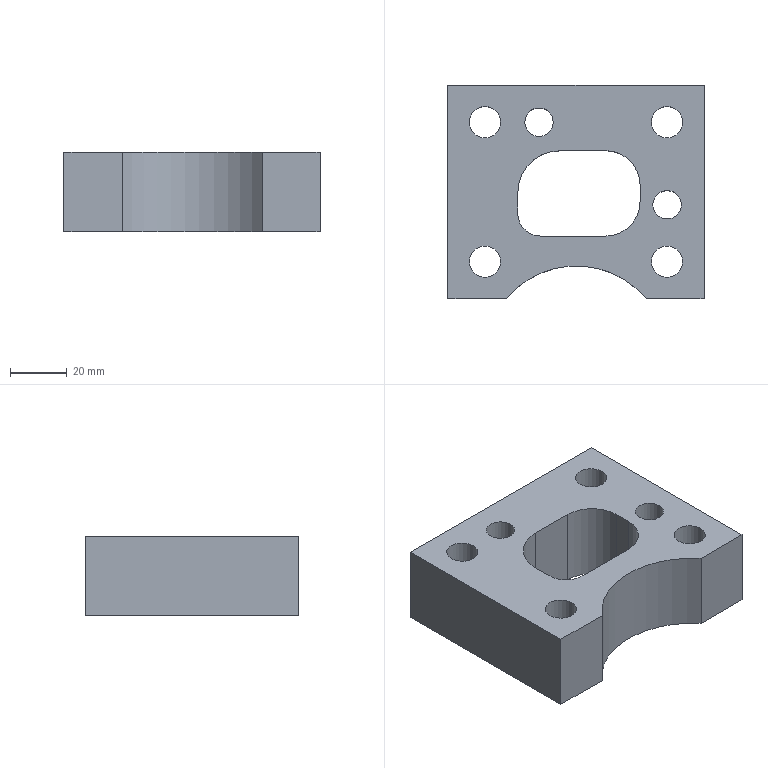Part | STEP file | PN_0017_id886_x_t | 1 solid | 30 faces | box 90 x 75 x 28 mm | volume 120807 mm3 | plane 15 | cylinder 15 | commonest cylinder face diameters 11 x4 17 x4 10 x2 24 x2 16 x1 30 x1
STEP:
#1=CARTESIAN_POINT('',(-240.086,-141.5,67.));
#2=VERTEX_POINT('',#1);
#3=CARTESIAN_POINT('',(-219.571,-141.5,67.));
#4=VERTEX_POINT('',#3);
#5=CARTESIAN_POINT('',(-207.586,-141.5,67.));
#6=DIRECTION('',(1.,0.,0.));
#7=VECTOR('',#6,1.);
#8=LINE('',#5,#7);
#9=EDGE_CURVE('',#2,#4,#8,.T.);
#10=ORIENTED_EDGE('',*,*,#9,.T.);
#11=CARTESIAN_POINT('',(-219.571,-141.5,95.));
#12=VERTEX_POINT('',#11);
#13=CARTESIAN_POINT('',(-219.571,-141.5,96.5));
#14=DIRECTION('',(0.,0.,-1.));
#15=VECTOR('',#14,1.);
#16=LINE('',#13,#15);
#17=EDGE_CURVE('',#12,#4,#16,.T.);
#18=ORIENTED_EDGE('',*,*,#17,.F.);
#19=CARTESIAN_POINT('',(-240.086,-141.5,95.));
#20=VERTEX_POINT('',#19);
#21=CARTESIAN_POINT('',(-207.586,-141.5,95.));
#22=DIRECTION('',(-1.,0.,0.));
#23=VECTOR('',#22,1.);
#24=LINE('',#21,#23);
#25=EDGE_CURVE('',#12,#20,#24,.T.);
#26=ORIENTED_EDGE('',*,*,#25,.T.);
#27=CARTESIAN_POINT('',(-240.086,-141.5,77.));
#28=DIRECTION('',(0.,0.,1.));
#29=VECTOR('',#28,1.);
#30=LINE('',#27,#29);
#31=EDGE_CURVE('',#2,#20,#30,.T.);
#32=ORIENTED_EDGE('',*,*,#31,.F.);
#33=EDGE_LOOP('',(#10,#18,#26,#32));
#34=FACE_OUTER_BOUND('',#33,.T.);
#35=CARTESIAN_POINT('',(-207.586,-141.5,77.));
#36=DIRECTION('',(0.,-1.,0.));
#37=DIRECTION('',(0.,0.,-1.));
#38=AXIS2_PLACEMENT_3D('',#35,#36,#37);
#39=PLANE('',#38);
#40=ADVANCED_FACE('',(#34),#39,.T.);
#41=CARTESIAN_POINT('',(-221.586,-79.5,95.));
#42=VERTEX_POINT('',#41);
#43=CARTESIAN_POINT('',(-227.086,-79.5,95.));
#44=DIRECTION('',(0.,0.,1.));
#45=DIRECTION('',(1.,0.,0.));
#46=AXIS2_PLACEMENT_3D('',#43,#44,#45);
#47=CIRCLE('',#46,5.5);
#48=EDGE_CURVE('',#42,#42,#47,.T.);
#49=ORIENTED_EDGE('',*,*,#48,.F.);
#50=EDGE_LOOP('',(#49));
#51=FACE_BOUND('',#50,.T.);
#52=CARTESIAN_POINT('',(-157.586,-79.5,95.));
#53=VERTEX_POINT('',#52);
#54=CARTESIAN_POINT('',(-163.086,-79.5,95.));
#55=DIRECTION('',(0.,0.,1.));
#56=DIRECTION('',(1.,0.,0.));
#57=AXIS2_PLACEMENT_3D('',#54,#55,#56);
#58=CIRCLE('',#57,5.5);
#59=EDGE_CURVE('',#53,#53,#58,.T.);
#60=ORIENTED_EDGE('',*,*,#59,.F.);
#61=EDGE_LOOP('',(#60));
#62=FACE_BOUND('',#61,.T.);
#63=CARTESIAN_POINT('',(-221.586,-128.5,95.));
#64=VERTEX_POINT('',#63);
#65=CARTESIAN_POINT('',(-227.086,-128.5,95.));
#66=DIRECTION('',(0.,0.,1.));
#67=DIRECTION('',(1.,0.,0.));
#68=AXIS2_PLACEMENT_3D('',#65,#66,#67);
#69=CIRCLE('',#68,5.5);
#70=EDGE_CURVE('',#64,#64,#69,.T.);
#71=ORIENTED_EDGE('',*,*,#70,.F.);
#72=EDGE_LOOP('',(#71));
#73=FACE_BOUND('',#72,.T.);
#74=CARTESIAN_POINT('',(-157.586,-128.5,95.));
#75=VERTEX_POINT('',#74);
#76=CARTESIAN_POINT('',(-163.086,-128.5,95.));
#77=DIRECTION('',(0.,0.,1.));
#78=DIRECTION('',(1.,0.,0.));
#79=AXIS2_PLACEMENT_3D('',#76,#77,#78);
#80=CIRCLE('',#79,5.5);
#81=EDGE_CURVE('',#75,#75,#80,.T.);
#82=ORIENTED_EDGE('',*,*,#81,.F.);
#83=EDGE_LOOP('',(#82));
#84=FACE_BOUND('',#83,.T.);
#85=CARTESIAN_POINT('',(-170.429,-141.5,95.));
#86=VERTEX_POINT('',#85);
#87=CARTESIAN_POINT('',(-195.,-162.,95.));
#88=DIRECTION('',(0.,0.,1.));
#89=DIRECTION('',(1.,0.,0.));
#90=AXIS2_PLACEMENT_3D('',#87,#88,#89);
#91=CIRCLE('',#90,32.);
#92=EDGE_CURVE('',#86,#12,#91,.T.);
#93=ORIENTED_EDGE('',*,*,#92,.F.);
#94=CARTESIAN_POINT('',(-150.086,-141.5,95.));
#95=VERTEX_POINT('',#94);
#96=CARTESIAN_POINT('',(-207.586,-141.5,95.));
#97=DIRECTION('',(-1.,0.,0.));
#98=VECTOR('',#97,1.);
#99=LINE('',#96,#98);
#100=EDGE_CURVE('',#95,#86,#99,.T.);
#101=ORIENTED_EDGE('',*,*,#100,.F.);
#102=CARTESIAN_POINT('',(-150.086,-66.5,95.));
#103=VERTEX_POINT('',#102);
#104=CARTESIAN_POINT('',(-150.086,-99.,95.));
#105=DIRECTION('',(0.,-1.,0.));
#106=VECTOR('',#105,1.);
#107=LINE('',#104,#106);
#108=EDGE_CURVE('',#103,#95,#107,.T.);
#109=ORIENTED_EDGE('',*,*,#108,.F.);
#110=CARTESIAN_POINT('',(-240.086,-66.5,95.));
#111=VERTEX_POINT('',#110);
#112=CARTESIAN_POINT('',(-207.586,-66.5,95.));
#113=DIRECTION('',(1.,0.,0.));
#114=VECTOR('',#113,1.);
#115=LINE('',#112,#114);
#116=EDGE_CURVE('',#111,#103,#115,.T.);
#117=ORIENTED_EDGE('',*,*,#116,.F.);
#118=CARTESIAN_POINT('',(-240.086,-99.,95.));
#119=DIRECTION('',(0.,1.,0.));
#120=VECTOR('',#119,1.);
#121=LINE('',#118,#120);
#122=EDGE_CURVE('',#20,#111,#121,.T.);
#123=ORIENTED_EDGE('',*,*,#122,.F.);
#124=ORIENTED_EDGE('',*,*,#25,.F.);
#125=EDGE_LOOP('',(#93,#101,#109,#117,#123,#124));
#126=FACE_BOUND('',#125,.T.);
#127=CARTESIAN_POINT('',(-184.586,-119.5,95.));
#128=VERTEX_POINT('',#127);
#129=CARTESIAN_POINT('',(-172.586,-107.5,95.));
#130=VERTEX_POINT('',#129);
#131=CARTESIAN_POINT('',(-184.586,-107.5,95.));
#132=DIRECTION('',(0.,0.,1.));
#133=DIRECTION('',(-1.,0.,0.));
#134=AXIS2_PLACEMENT_3D('',#131,#132,#133);
#135=CIRCLE('',#134,12.);
#136=EDGE_CURVE('',#128,#130,#135,.T.);
#137=ORIENTED_EDGE('',*,*,#136,.F.);
#138=CARTESIAN_POINT('',(-207.586,-119.5,95.));
#139=VERTEX_POINT('',#138);
#140=CARTESIAN_POINT('',(-211.586,-119.5,95.));
#141=DIRECTION('',(1.,0.,0.));
#142=VECTOR('',#141,1.);
#143=LINE('',#140,#142);
#144=EDGE_CURVE('',#139,#128,#143,.T.);
#145=ORIENTED_EDGE('',*,*,#144,.F.);
#146=CARTESIAN_POINT('',(-215.586,-111.5,95.));
#147=VERTEX_POINT('',#146);
#148=CARTESIAN_POINT('',(-207.586,-111.5,95.));
#149=DIRECTION('',(0.,0.,1.));
#150=DIRECTION('',(-1.,0.,0.));
#151=AXIS2_PLACEMENT_3D('',#148,#149,#150);
#152=CIRCLE('',#151,8.);
#153=EDGE_CURVE('',#147,#139,#152,.T.);
#154=ORIENTED_EDGE('',*,*,#153,.F.);
#155=CARTESIAN_POINT('',(-215.586,-104.5,95.));
#156=VERTEX_POINT('',#155);
#157=CARTESIAN_POINT('',(-215.586,-80.,95.));
#158=DIRECTION('',(0.,-1.,0.));
#159=VECTOR('',#158,1.);
#160=LINE('',#157,#159);
#161=EDGE_CURVE('',#156,#147,#160,.T.);
#162=ORIENTED_EDGE('',*,*,#161,.F.);
#163=CARTESIAN_POINT('',(-200.586,-89.5,95.));
#164=VERTEX_POINT('',#163);
#165=CARTESIAN_POINT('',(-200.586,-104.5,95.));
#166=DIRECTION('',(0.,0.,1.));
#167=DIRECTION('',(-1.,0.,0.));
#168=AXIS2_PLACEMENT_3D('',#165,#166,#167);
#169=CIRCLE('',#168,15.);
#170=EDGE_CURVE('',#164,#156,#169,.T.);
#171=ORIENTED_EDGE('',*,*,#170,.F.);
#172=CARTESIAN_POINT('',(-184.586,-89.5,95.));
#173=VERTEX_POINT('',#172);
#174=CARTESIAN_POINT('',(-189.586,-89.5,95.));
#175=DIRECTION('',(-1.,0.,0.));
#176=VECTOR('',#175,1.);
#177=LINE('',#174,#176);
#178=EDGE_CURVE('',#173,#164,#177,.T.);
#179=ORIENTED_EDGE('',*,*,#178,.F.);
#180=CARTESIAN_POINT('',(-172.586,-101.5,95.));
#181=VERTEX_POINT('',#180);
#182=CARTESIAN_POINT('',(-184.586,-101.5,95.));
#183=DIRECTION('',(0.,0.,1.));
#184=DIRECTION('',(-1.,0.,0.));
#185=AXIS2_PLACEMENT_3D('',#182,#183,#184);
#186=CIRCLE('',#185,12.);
#187=EDGE_CURVE('',#181,#173,#186,.T.);
#188=ORIENTED_EDGE('',*,*,#187,.F.);
#189=CARTESIAN_POINT('',(-172.586,-115.,95.));
#190=DIRECTION('',(0.,1.,0.));
#191=VECTOR('',#190,1.);
#192=LINE('',#189,#191);
#193=EDGE_CURVE('',#130,#181,#192,.T.);
#194=ORIENTED_EDGE('',*,*,#193,.F.);
#195=EDGE_LOOP('',(#137,#145,#154,#162,#171,#179,#188,#194));
#196=FACE_BOUND('',#195,.T.);
#197=CARTESIAN_POINT('',(-168.086,-108.5,95.));
#198=VERTEX_POINT('',#197);
#199=CARTESIAN_POINT('',(-163.086,-108.5,95.));
#200=DIRECTION('',(0.,0.,1.));
#201=DIRECTION('',(-1.,0.,0.));
#202=AXIS2_PLACEMENT_3D('',#199,#200,#201);
#203=CIRCLE('',#202,5.);
#204=EDGE_CURVE('',#198,#198,#203,.T.);
#205=ORIENTED_EDGE('',*,*,#204,.F.);
#206=EDGE_LOOP('',(#205));
#207=FACE_BOUND('',#206,.T.);
#208=CARTESIAN_POINT('',(-203.086,-79.5,95.));
#209=VERTEX_POINT('',#208);
#210=CARTESIAN_POINT('',(-208.086,-79.5,95.));
#211=DIRECTION('',(0.,0.,1.));
#212=DIRECTION('',(1.,0.,0.));
#213=AXIS2_PLACEMENT_3D('',#210,#211,#212);
#214=CIRCLE('',#213,5.);
#215=EDGE_CURVE('',#209,#209,#214,.T.);
#216=ORIENTED_EDGE('',*,*,#215,.F.);
#217=EDGE_LOOP('',(#216));
#218=FACE_BOUND('',#217,.T.);
#219=CARTESIAN_POINT('',(-119.811,64.,95.));
#220=DIRECTION('',(0.,0.,1.));
#221=DIRECTION('',(1.,0.,0.));
#222=AXIS2_PLACEMENT_3D('',#219,#220,#221);
#223=PLANE('',#222);
#224=ADVANCED_FACE('',(#51,#62,#73,#84,#126,#196,#207,#218),#223,.T.);
#225=CARTESIAN_POINT('',(-170.429,-141.5,67.));
#226=VERTEX_POINT('',#225);
#227=CARTESIAN_POINT('',(-170.429,-141.5,96.5));
#228=DIRECTION('',(0.,0.,1.));
#229=VECTOR('',#228,1.);
#230=LINE('',#227,#229);
#231=EDGE_CURVE('',#226,#86,#230,.T.);
#232=ORIENTED_EDGE('',*,*,#231,.F.);
#233=CARTESIAN_POINT('',(-150.086,-141.5,67.));
#234=VERTEX_POINT('',#233);
#235=CARTESIAN_POINT('',(-207.586,-141.5,67.));
#236=DIRECTION('',(1.,0.,0.));
#237=VECTOR('',#236,1.);
#238=LINE('',#235,#237);
#239=EDGE_CURVE('',#226,#234,#238,.T.);
#240=ORIENTED_EDGE('',*,*,#239,.T.);
#241=CARTESIAN_POINT('',(-150.086,-141.5,77.));
#242=DIRECTION('',(0.,0.,1.));
#243=VECTOR('',#242,1.);
#244=LINE('',#241,#243);
#245=EDGE_CURVE('',#234,#95,#244,.T.);
#246=ORIENTED_EDGE('',*,*,#245,.T.);
#247=ORIENTED_EDGE('',*,*,#100,.T.);
#248=EDGE_LOOP('',(#232,#240,#246,#247));
#249=FACE_OUTER_BOUND('',#248,.T.);
#250=CARTESIAN_POINT('',(-207.586,-141.5,77.));
#251=DIRECTION('',(0.,-1.,0.));
#252=DIRECTION('',(0.,0.,-1.));
#253=AXIS2_PLACEMENT_3D('',#250,#251,#252);
#254=PLANE('',#253);
#255=ADVANCED_FACE('',(#249),#254,.T.);
#256=ORIENTED_EDGE('',*,*,#31,.T.);
#257=ORIENTED_EDGE('',*,*,#122,.T.);
#258=CARTESIAN_POINT('',(-240.086,-66.5,67.));
#259=VERTEX_POINT('',#258);
#260=CARTESIAN_POINT('',(-240.086,-66.5,77.));
#261=DIRECTION('',(0.,0.,1.));
#262=VECTOR('',#261,1.);
#263=LINE('',#260,#262);
#264=EDGE_CURVE('',#259,#111,#263,.T.);
#265=ORIENTED_EDGE('',*,*,#264,.F.);
#266=CARTESIAN_POINT('',(-240.086,-99.,67.));
#267=DIRECTION('',(0.,-1.,0.));
#268=VECTOR('',#267,1.);
#269=LINE('',#266,#268);
#270=EDGE_CURVE('',#259,#2,#269,.T.);
#271=ORIENTED_EDGE('',*,*,#270,.T.);
#272=EDGE_LOOP('',(#256,#257,#265,#271));
#273=FACE_OUTER_BOUND('',#272,.T.);
#274=CARTESIAN_POINT('',(-240.086,-99.,77.));
#275=DIRECTION('',(-1.,0.,0.));
#276=DIRECTION('',(0.,0.,1.));
#277=AXIS2_PLACEMENT_3D('',#274,#275,#276);
#278=PLANE('',#277);
#279=ADVANCED_FACE('',(#273),#278,.T.);
#280=ORIENTED_EDGE('',*,*,#264,.T.);
#281=ORIENTED_EDGE('',*,*,#116,.T.);
#282=CARTESIAN_POINT('',(-150.086,-66.5,67.));
#283=VERTEX_POINT('',#282);
#284=CARTESIAN_POINT('',(-150.086,-66.5,77.));
#285=DIRECTION('',(0.,0.,1.));
#286=VECTOR('',#285,1.);
#287=LINE('',#284,#286);
#288=EDGE_CURVE('',#283,#103,#287,.T.);
#289=ORIENTED_EDGE('',*,*,#288,.F.);
#290=CARTESIAN_POINT('',(-207.586,-66.5,67.));
#291=DIRECTION('',(-1.,0.,0.));
#292=VECTOR('',#291,1.);
#293=LINE('',#290,#292);
#294=EDGE_CURVE('',#283,#259,#293,.T.);
#295=ORIENTED_EDGE('',*,*,#294,.T.);
#296=EDGE_LOOP('',(#280,#281,#289,#295));
#297=FACE_OUTER_BOUND('',#296,.T.);
#298=CARTESIAN_POINT('',(-207.586,-66.5,77.));
#299=DIRECTION('',(0.,1.,0.));
#300=DIRECTION('',(0.,0.,1.));
#301=AXIS2_PLACEMENT_3D('',#298,#299,#300);
#302=PLANE('',#301);
#303=ADVANCED_FACE('',(#297),#302,.T.);
#304=CARTESIAN_POINT('',(-235.586,-79.5,67.));
#305=VERTEX_POINT('',#304);
#306=CARTESIAN_POINT('',(-227.086,-79.5,67.));
#307=DIRECTION('',(0.,0.,-1.));
#308=DIRECTION('',(-1.,0.,0.));
#309=AXIS2_PLACEMENT_3D('',#306,#307,#308);
#310=CIRCLE('',#309,8.5);
#311=EDGE_CURVE('',#305,#305,#310,.T.);
#312=ORIENTED_EDGE('',*,*,#311,.F.);
#313=EDGE_LOOP('',(#312));
#314=FACE_BOUND('',#313,.T.);
#315=CARTESIAN_POINT('',(-203.086,-79.5,67.));
#316=VERTEX_POINT('',#315);
#317=CARTESIAN_POINT('',(-208.086,-79.5,67.));
#318=DIRECTION('',(0.,0.,1.));
#319=DIRECTION('',(1.,0.,0.));
#320=AXIS2_PLACEMENT_3D('',#317,#318,#319);
#321=CIRCLE('',#320,5.);
#322=EDGE_CURVE('',#316,#316,#321,.T.);
#323=ORIENTED_EDGE('',*,*,#322,.T.);
#324=EDGE_LOOP('',(#323));
#325=FACE_BOUND('',#324,.T.);
#326=CARTESIAN_POINT('',(-154.586,-79.5,67.));
#327=VERTEX_POINT('',#326);
#328=CARTESIAN_POINT('',(-163.086,-79.5,67.));
#329=DIRECTION('',(0.,0.,1.));
#330=DIRECTION('',(1.,0.,0.));
#331=AXIS2_PLACEMENT_3D('',#328,#329,#330);
#332=CIRCLE('',#331,8.5);
#333=EDGE_CURVE('',#327,#327,#332,.T.);
#334=ORIENTED_EDGE('',*,*,#333,.T.);
#335=EDGE_LOOP('',(#334));
#336=FACE_BOUND('',#335,.T.);
#337=CARTESIAN_POINT('',(-235.586,-128.5,67.));
#338=VERTEX_POINT('',#337);
#339=CARTESIAN_POINT('',(-227.086,-128.5,67.));
#340=DIRECTION('',(0.,0.,1.));
#341=DIRECTION('',(-1.,0.,0.));
#342=AXIS2_PLACEMENT_3D('',#339,#340,#341);
#343=CIRCLE('',#342,8.5);
#344=EDGE_CURVE('',#338,#338,#343,.T.);
#345=ORIENTED_EDGE('',*,*,#344,.T.);
#346=EDGE_LOOP('',(#345));
#347=FACE_BOUND('',#346,.T.);
#348=CARTESIAN_POINT('',(-168.086,-108.5,67.));
#349=VERTEX_POINT('',#348);
#350=CARTESIAN_POINT('',(-163.086,-108.5,67.));
#351=DIRECTION('',(0.,0.,1.));
#352=DIRECTION('',(-1.,0.,0.));
#353=AXIS2_PLACEMENT_3D('',#350,#351,#352);
#354=CIRCLE('',#353,5.);
#355=EDGE_CURVE('',#349,#349,#354,.T.);
#356=ORIENTED_EDGE('',*,*,#355,.T.);
#357=EDGE_LOOP('',(#356));
#358=FACE_BOUND('',#357,.T.);
#359=CARTESIAN_POINT('',(-154.586,-128.5,67.));
#360=VERTEX_POINT('',#359);
#361=CARTESIAN_POINT('',(-163.086,-128.5,67.));
#362=DIRECTION('',(0.,0.,-1.));
#363=DIRECTION('',(1.,0.,0.));
#364=AXIS2_PLACEMENT_3D('',#361,#362,#363);
#365=CIRCLE('',#364,8.5);
#366=EDGE_CURVE('',#360,#360,#365,.T.);
#367=ORIENTED_EDGE('',*,*,#366,.F.);
#368=EDGE_LOOP('',(#367));
#369=FACE_BOUND('',#368,.T.);
#370=CARTESIAN_POINT('',(-184.586,-89.5,67.));
#371=VERTEX_POINT('',#370);
#372=CARTESIAN_POINT('',(-172.586,-101.5,67.));
#373=VERTEX_POINT('',#372);
#374=CARTESIAN_POINT('',(-184.586,-101.5,67.));
#375=DIRECTION('',(0.,0.,-1.));
#376=DIRECTION('',(1.,0.,0.));
#377=AXIS2_PLACEMENT_3D('',#374,#375,#376);
#378=CIRCLE('',#377,12.);
#379=EDGE_CURVE('',#371,#373,#378,.T.);
#380=ORIENTED_EDGE('',*,*,#379,.F.);
#381=CARTESIAN_POINT('',(-200.586,-89.5,67.));
#382=VERTEX_POINT('',#381);
#383=CARTESIAN_POINT('',(-119.811,-89.5,67.));
#384=DIRECTION('',(-1.,0.,0.));
#385=VECTOR('',#384,1.);
#386=LINE('',#383,#385);
#387=EDGE_CURVE('',#371,#382,#386,.T.);
#388=ORIENTED_EDGE('',*,*,#387,.T.);
#389=CARTESIAN_POINT('',(-215.586,-104.5,67.));
#390=VERTEX_POINT('',#389);
#391=CARTESIAN_POINT('',(-200.586,-104.5,67.));
#392=DIRECTION('',(0.,0.,-1.));
#393=DIRECTION('',(1.,0.,0.));
#394=AXIS2_PLACEMENT_3D('',#391,#392,#393);
#395=CIRCLE('',#394,15.);
#396=EDGE_CURVE('',#390,#382,#395,.T.);
#397=ORIENTED_EDGE('',*,*,#396,.F.);
#398=CARTESIAN_POINT('',(-215.586,-111.5,67.));
#399=VERTEX_POINT('',#398);
#400=CARTESIAN_POINT('',(-215.586,64.,67.));
#401=DIRECTION('',(0.,-1.,0.));
#402=VECTOR('',#401,1.);
#403=LINE('',#400,#402);
#404=EDGE_CURVE('',#390,#399,#403,.T.);
#405=ORIENTED_EDGE('',*,*,#404,.T.);
#406=CARTESIAN_POINT('',(-207.586,-119.5,67.));
#407=VERTEX_POINT('',#406);
#408=CARTESIAN_POINT('',(-207.586,-111.5,67.));
#409=DIRECTION('',(0.,0.,-1.));
#410=DIRECTION('',(1.,0.,0.));
#411=AXIS2_PLACEMENT_3D('',#408,#409,#410);
#412=CIRCLE('',#411,8.);
#413=EDGE_CURVE('',#407,#399,#412,.T.);
#414=ORIENTED_EDGE('',*,*,#413,.F.);
#415=CARTESIAN_POINT('',(-184.586,-119.5,67.));
#416=VERTEX_POINT('',#415);
#417=CARTESIAN_POINT('',(-119.811,-119.5,67.));
#418=DIRECTION('',(1.,0.,0.));
#419=VECTOR('',#418,1.);
#420=LINE('',#417,#419);
#421=EDGE_CURVE('',#407,#416,#420,.T.);
#422=ORIENTED_EDGE('',*,*,#421,.T.);
#423=CARTESIAN_POINT('',(-172.586,-107.5,67.));
#424=VERTEX_POINT('',#423);
#425=CARTESIAN_POINT('',(-184.586,-107.5,67.));
#426=DIRECTION('',(0.,0.,-1.));
#427=DIRECTION('',(1.,0.,0.));
#428=AXIS2_PLACEMENT_3D('',#425,#426,#427);
#429=CIRCLE('',#428,12.);
#430=EDGE_CURVE('',#424,#416,#429,.T.);
#431=ORIENTED_EDGE('',*,*,#430,.F.);
#432=CARTESIAN_POINT('',(-172.586,64.,67.));
#433=DIRECTION('',(0.,1.,0.));
#434=VECTOR('',#433,1.);
#435=LINE('',#432,#434);
#436=EDGE_CURVE('',#424,#373,#435,.T.);
#437=ORIENTED_EDGE('',*,*,#436,.T.);
#438=EDGE_LOOP('',(#380,#388,#397,#405,#414,#422,#431,#437));
#439=FACE_BOUND('',#438,.T.);
#440=ORIENTED_EDGE('',*,*,#239,.F.);
#441=CARTESIAN_POINT('',(-195.,-162.,67.));
#442=DIRECTION('',(0.,0.,1.));
#443=DIRECTION('',(1.,0.,0.));
#444=AXIS2_PLACEMENT_3D('',#441,#442,#443);
#445=CIRCLE('',#444,32.);
#446=EDGE_CURVE('',#226,#4,#445,.T.);
#447=ORIENTED_EDGE('',*,*,#446,.T.);
#448=ORIENTED_EDGE('',*,*,#9,.F.);
#449=ORIENTED_EDGE('',*,*,#270,.F.);
#450=ORIENTED_EDGE('',*,*,#294,.F.);
#451=CARTESIAN_POINT('',(-150.086,-99.,67.));
#452=DIRECTION('',(0.,1.,0.));
#453=VECTOR('',#452,1.);
#454=LINE('',#451,#453);
#455=EDGE_CURVE('',#234,#283,#454,.T.);
#456=ORIENTED_EDGE('',*,*,#455,.F.);
#457=EDGE_LOOP('',(#440,#447,#448,#449,#450,#456));
#458=FACE_BOUND('',#457,.T.);
#459=CARTESIAN_POINT('',(-119.811,64.,67.));
#460=DIRECTION('',(0.,0.,1.));
#461=DIRECTION('',(1.,0.,0.));
#462=AXIS2_PLACEMENT_3D('',#459,#460,#461);
#463=PLANE('',#462);
#464=ADVANCED_FACE('',(#314,#325,#336,#347,#358,#369,#439,#458),#463,.F.);
#465=ORIENTED_EDGE('',*,*,#455,.T.);
#466=ORIENTED_EDGE('',*,*,#288,.T.);
#467=ORIENTED_EDGE('',*,*,#108,.T.);
#468=ORIENTED_EDGE('',*,*,#245,.F.);
#469=EDGE_LOOP('',(#465,#466,#467,#468));
#470=FACE_OUTER_BOUND('',#469,.T.);
#471=CARTESIAN_POINT('',(-150.086,-99.,77.));
#472=DIRECTION('',(1.,0.,0.));
#473=DIRECTION('',(0.,0.,-1.));
#474=AXIS2_PLACEMENT_3D('',#471,#472,#473);
#475=PLANE('',#474);
#476=ADVANCED_FACE('',(#470),#475,.T.);
#477=ORIENTED_EDGE('',*,*,#396,.T.);
#478=CARTESIAN_POINT('',(-200.586,-89.5,78.6));
#479=DIRECTION('',(0.,0.,-1.));
#480=VECTOR('',#479,1.);
#481=LINE('',#478,#480);
#482=EDGE_CURVE('',#164,#382,#481,.T.);
#483=ORIENTED_EDGE('',*,*,#482,.F.);
#484=ORIENTED_EDGE('',*,*,#170,.T.);
#485=CARTESIAN_POINT('',(-215.586,-104.5,78.6));
#486=DIRECTION('',(0.,0.,1.));
#487=VECTOR('',#486,1.);
#488=LINE('',#485,#487);
#489=EDGE_CURVE('',#390,#156,#488,.T.);
#490=ORIENTED_EDGE('',*,*,#489,.F.);
#491=EDGE_LOOP('',(#477,#483,#484,#490));
#492=FACE_OUTER_BOUND('',#491,.T.);
#493=CARTESIAN_POINT('',(-200.586,-104.5,78.6));
#494=DIRECTION('',(0.,0.,-1.));
#495=DIRECTION('',(-1.,0.,0.));
#496=AXIS2_PLACEMENT_3D('',#493,#494,#495);
#497=CYLINDRICAL_SURFACE('',#496,15.);
#498=ADVANCED_FACE('',(#492),#497,.F.);
#499=ORIENTED_EDGE('',*,*,#379,.T.);
#500=CARTESIAN_POINT('',(-172.586,-101.5,78.6));
#501=DIRECTION('',(0.,0.,-1.));
#502=VECTOR('',#501,1.);
#503=LINE('',#500,#502);
#504=EDGE_CURVE('',#181,#373,#503,.T.);
#505=ORIENTED_EDGE('',*,*,#504,.F.);
#506=ORIENTED_EDGE('',*,*,#187,.T.);
#507=CARTESIAN_POINT('',(-184.586,-89.5,78.6));
#508=DIRECTION('',(0.,0.,1.));
#509=VECTOR('',#508,1.);
#510=LINE('',#507,#509);
#511=EDGE_CURVE('',#371,#173,#510,.T.);
#512=ORIENTED_EDGE('',*,*,#511,.F.);
#513=EDGE_LOOP('',(#499,#505,#506,#512));
#514=FACE_OUTER_BOUND('',#513,.T.);
#515=CARTESIAN_POINT('',(-184.586,-101.5,78.6));
#516=DIRECTION('',(0.,0.,-1.));
#517=DIRECTION('',(-1.,0.,0.));
#518=AXIS2_PLACEMENT_3D('',#515,#516,#517);
#519=CYLINDRICAL_SURFACE('',#518,12.);
#520=ADVANCED_FACE('',(#514),#519,.F.);
#521=ORIENTED_EDGE('',*,*,#511,.T.);
#522=ORIENTED_EDGE('',*,*,#178,.T.);
#523=ORIENTED_EDGE('',*,*,#482,.T.);
#524=ORIENTED_EDGE('',*,*,#387,.F.);
#525=EDGE_LOOP('',(#521,#522,#523,#524));
#526=FACE_OUTER_BOUND('',#525,.T.);
#527=CARTESIAN_POINT('',(-189.586,-89.5,78.6));
#528=DIRECTION('',(0.,-1.,0.));
#529=DIRECTION('',(0.,0.,-1.));
#530=AXIS2_PLACEMENT_3D('',#527,#528,#529);
#531=PLANE('',#530);
#532=ADVANCED_FACE('',(#526),#531,.T.);
#533=ORIENTED_EDGE('',*,*,#430,.T.);
#534=CARTESIAN_POINT('',(-184.586,-119.5,78.6));
#535=DIRECTION('',(0.,0.,-1.));
#536=VECTOR('',#535,1.);
#537=LINE('',#534,#536);
#538=EDGE_CURVE('',#128,#416,#537,.T.);
#539=ORIENTED_EDGE('',*,*,#538,.F.);
#540=ORIENTED_EDGE('',*,*,#136,.T.);
#541=CARTESIAN_POINT('',(-172.586,-107.5,78.6));
#542=DIRECTION('',(0.,0.,1.));
#543=VECTOR('',#542,1.);
#544=LINE('',#541,#543);
#545=EDGE_CURVE('',#424,#130,#544,.T.);
#546=ORIENTED_EDGE('',*,*,#545,.F.);
#547=EDGE_LOOP('',(#533,#539,#540,#546));
#548=FACE_OUTER_BOUND('',#547,.T.);
#549=CARTESIAN_POINT('',(-184.586,-107.5,78.6));
#550=DIRECTION('',(0.,0.,-1.));
#551=DIRECTION('',(-1.,0.,0.));
#552=AXIS2_PLACEMENT_3D('',#549,#550,#551);
#553=CYLINDRICAL_SURFACE('',#552,12.);
#554=ADVANCED_FACE('',(#548),#553,.F.);
#555=ORIENTED_EDGE('',*,*,#545,.T.);
#556=ORIENTED_EDGE('',*,*,#193,.T.);
#557=ORIENTED_EDGE('',*,*,#504,.T.);
#558=ORIENTED_EDGE('',*,*,#436,.F.);
#559=EDGE_LOOP('',(#555,#556,#557,#558));
#560=FACE_OUTER_BOUND('',#559,.T.);
#561=CARTESIAN_POINT('',(-172.586,-115.,78.6));
#562=DIRECTION('',(-1.,0.,0.));
#563=DIRECTION('',(0.,0.,1.));
#564=AXIS2_PLACEMENT_3D('',#561,#562,#563);
#565=PLANE('',#564);
#566=ADVANCED_FACE('',(#560),#565,.T.);
#567=ORIENTED_EDGE('',*,*,#413,.T.);
#568=CARTESIAN_POINT('',(-215.586,-111.5,78.6));
#569=DIRECTION('',(0.,0.,-1.));
#570=VECTOR('',#569,1.);
#571=LINE('',#568,#570);
#572=EDGE_CURVE('',#147,#399,#571,.T.);
#573=ORIENTED_EDGE('',*,*,#572,.F.);
#574=ORIENTED_EDGE('',*,*,#153,.T.);
#575=CARTESIAN_POINT('',(-207.586,-119.5,78.6));
#576=DIRECTION('',(0.,0.,1.));
#577=VECTOR('',#576,1.);
#578=LINE('',#575,#577);
#579=EDGE_CURVE('',#407,#139,#578,.T.);
#580=ORIENTED_EDGE('',*,*,#579,.F.);
#581=EDGE_LOOP('',(#567,#573,#574,#580));
#582=FACE_OUTER_BOUND('',#581,.T.);
#583=CARTESIAN_POINT('',(-207.586,-111.5,78.6));
#584=DIRECTION('',(0.,0.,1.));
#585=DIRECTION('',(1.,0.,0.));
#586=AXIS2_PLACEMENT_3D('',#583,#584,#585);
#587=CYLINDRICAL_SURFACE('',#586,8.);
#588=ADVANCED_FACE('',(#582),#587,.F.);
#589=ORIENTED_EDGE('',*,*,#579,.T.);
#590=ORIENTED_EDGE('',*,*,#144,.T.);
#591=ORIENTED_EDGE('',*,*,#538,.T.);
#592=ORIENTED_EDGE('',*,*,#421,.F.);
#593=EDGE_LOOP('',(#589,#590,#591,#592));
#594=FACE_OUTER_BOUND('',#593,.T.);
#595=CARTESIAN_POINT('',(-211.586,-119.5,78.6));
#596=DIRECTION('',(0.,1.,0.));
#597=DIRECTION('',(0.,0.,1.));
#598=AXIS2_PLACEMENT_3D('',#595,#596,#597);
#599=PLANE('',#598);
#600=ADVANCED_FACE('',(#594),#599,.T.);
#601=ORIENTED_EDGE('',*,*,#489,.T.);
#602=ORIENTED_EDGE('',*,*,#161,.T.);
#603=ORIENTED_EDGE('',*,*,#572,.T.);
#604=ORIENTED_EDGE('',*,*,#404,.F.);
#605=EDGE_LOOP('',(#601,#602,#603,#604));
#606=FACE_OUTER_BOUND('',#605,.T.);
#607=CARTESIAN_POINT('',(-215.586,-80.,78.6));
#608=DIRECTION('',(1.,0.,0.));
#609=DIRECTION('',(0.,0.,-1.));
#610=AXIS2_PLACEMENT_3D('',#607,#608,#609);
#611=PLANE('',#610);
#612=ADVANCED_FACE('',(#606),#611,.T.);
#613=ORIENTED_EDGE('',*,*,#446,.F.);
#614=ORIENTED_EDGE('',*,*,#231,.T.);
#615=ORIENTED_EDGE('',*,*,#92,.T.);
#616=ORIENTED_EDGE('',*,*,#17,.T.);
#617=EDGE_LOOP('',(#613,#614,#615,#616));
#618=FACE_OUTER_BOUND('',#617,.T.);
#619=CARTESIAN_POINT('',(-195.,-162.,96.5));
#620=DIRECTION('',(0.,0.,-1.));
#621=DIRECTION('',(1.,0.,0.));
#622=AXIS2_PLACEMENT_3D('',#619,#620,#621);
#623=CYLINDRICAL_SURFACE('',#622,32.);
#624=ADVANCED_FACE('',(#618),#623,.F.);
#625=ORIENTED_EDGE('',*,*,#81,.T.);
#626=EDGE_LOOP('',(#625));
#627=FACE_BOUND('',#626,.T.);
#628=CARTESIAN_POINT('',(-157.586,-128.5,85.));
#629=VERTEX_POINT('',#628);
#630=CARTESIAN_POINT('',(-163.086,-128.5,85.));
#631=DIRECTION('',(0.,0.,-1.));
#632=DIRECTION('',(1.,0.,0.));
#633=AXIS2_PLACEMENT_3D('',#630,#631,#632);
#634=CIRCLE('',#633,5.5);
#635=EDGE_CURVE('',#629,#629,#634,.T.);
#636=ORIENTED_EDGE('',*,*,#635,.T.);
#637=EDGE_LOOP('',(#636));
#638=FACE_BOUND('',#637,.T.);
#639=CARTESIAN_POINT('',(-163.086,-128.5,105.));
#640=DIRECTION('',(0.,0.,-1.));
#641=DIRECTION('',(-1.,0.,0.));
#642=AXIS2_PLACEMENT_3D('',#639,#640,#641);
#643=CYLINDRICAL_SURFACE('',#642,5.5);
#644=ADVANCED_FACE('',(#627,#638),#643,.F.);
#645=ORIENTED_EDGE('',*,*,#635,.F.);
#646=EDGE_LOOP('',(#645));
#647=FACE_BOUND('',#646,.T.);
#648=CARTESIAN_POINT('',(-171.586,-128.5,85.));
#649=VERTEX_POINT('',#648);
#650=CARTESIAN_POINT('',(-163.086,-128.5,85.));
#651=DIRECTION('',(0.,0.,-1.));
#652=DIRECTION('',(-1.,0.,0.));
#653=AXIS2_PLACEMENT_3D('',#650,#651,#652);
#654=CIRCLE('',#653,8.5);
#655=EDGE_CURVE('',#649,#649,#654,.T.);
#656=ORIENTED_EDGE('',*,*,#655,.T.);
#657=EDGE_LOOP('',(#656));
#658=FACE_BOUND('',#657,.T.);
#659=CARTESIAN_POINT('',(-163.086,-128.5,85.));
#660=DIRECTION('',(0.,0.,1.));
#661=DIRECTION('',(1.,0.,0.));
#662=AXIS2_PLACEMENT_3D('',#659,#660,#661);
#663=PLANE('',#662);
#664=ADVANCED_FACE('',(#647,#658),#663,.F.);
#665=ORIENTED_EDGE('',*,*,#366,.T.);
#666=EDGE_LOOP('',(#665));
#667=FACE_BOUND('',#666,.T.);
#668=ORIENTED_EDGE('',*,*,#655,.F.);
#669=EDGE_LOOP('',(#668));
#670=FACE_BOUND('',#669,.T.);
#671=CARTESIAN_POINT('',(-163.086,-128.5,85.));
#672=DIRECTION('',(0.,0.,-1.));
#673=DIRECTION('',(-1.,0.,0.));
#674=AXIS2_PLACEMENT_3D('',#671,#672,#673);
#675=CYLINDRICAL_SURFACE('',#674,8.5);
#676=ADVANCED_FACE('',(#667,#670),#675,.F.);
#677=ORIENTED_EDGE('',*,*,#204,.T.);
#678=EDGE_LOOP('',(#677));
#679=FACE_BOUND('',#678,.T.);
#680=ORIENTED_EDGE('',*,*,#355,.F.);
#681=EDGE_LOOP('',(#680));
#682=FACE_BOUND('',#681,.T.);
#683=CARTESIAN_POINT('',(-163.086,-108.5,105.));
#684=DIRECTION('',(0.,0.,-1.));
#685=DIRECTION('',(-1.,0.,0.));
#686=AXIS2_PLACEMENT_3D('',#683,#684,#685);
#687=CYLINDRICAL_SURFACE('',#686,5.);
#688=ADVANCED_FACE('',(#679,#682),#687,.F.);
#689=ORIENTED_EDGE('',*,*,#70,.T.);
#690=EDGE_LOOP('',(#689));
#691=FACE_BOUND('',#690,.T.);
#692=CARTESIAN_POINT('',(-232.586,-128.5,85.));
#693=VERTEX_POINT('',#692);
#694=CARTESIAN_POINT('',(-227.086,-128.5,85.));
#695=DIRECTION('',(0.,0.,1.));
#696=DIRECTION('',(-1.,0.,0.));
#697=AXIS2_PLACEMENT_3D('',#694,#695,#696);
#698=CIRCLE('',#697,5.5);
#699=EDGE_CURVE('',#693,#693,#698,.T.);
#700=ORIENTED_EDGE('',*,*,#699,.F.);
#701=EDGE_LOOP('',(#700));
#702=FACE_BOUND('',#701,.T.);
#703=CARTESIAN_POINT('',(-227.086,-128.5,105.));
#704=DIRECTION('',(0.,0.,-1.));
#705=DIRECTION('',(1.,0.,0.));
#706=AXIS2_PLACEMENT_3D('',#703,#704,#705);
#707=CYLINDRICAL_SURFACE('',#706,5.5);
#708=ADVANCED_FACE('',(#691,#702),#707,.F.);
#709=ORIENTED_EDGE('',*,*,#699,.T.);
#710=EDGE_LOOP('',(#709));
#711=FACE_BOUND('',#710,.T.);
#712=CARTESIAN_POINT('',(-218.586,-128.5,85.));
#713=VERTEX_POINT('',#712);
#714=CARTESIAN_POINT('',(-227.086,-128.5,85.));
#715=DIRECTION('',(0.,0.,1.));
#716=DIRECTION('',(1.,0.,0.));
#717=AXIS2_PLACEMENT_3D('',#714,#715,#716);
#718=CIRCLE('',#717,8.5);
#719=EDGE_CURVE('',#713,#713,#718,.T.);
#720=ORIENTED_EDGE('',*,*,#719,.F.);
#721=EDGE_LOOP('',(#720));
#722=FACE_BOUND('',#721,.T.);
#723=CARTESIAN_POINT('',(-227.086,-128.5,85.));
#724=DIRECTION('',(0.,0.,1.));
#725=DIRECTION('',(-1.,0.,0.));
#726=AXIS2_PLACEMENT_3D('',#723,#724,#725);
#727=PLANE('',#726);
#728=ADVANCED_FACE('',(#711,#722),#727,.F.);
#729=ORIENTED_EDGE('',*,*,#344,.F.);
#730=EDGE_LOOP('',(#729));
#731=FACE_BOUND('',#730,.T.);
#732=ORIENTED_EDGE('',*,*,#719,.T.);
#733=EDGE_LOOP('',(#732));
#734=FACE_BOUND('',#733,.T.);
#735=CARTESIAN_POINT('',(-227.086,-128.5,85.));
#736=DIRECTION('',(0.,0.,-1.));
#737=DIRECTION('',(1.,0.,0.));
#738=AXIS2_PLACEMENT_3D('',#735,#736,#737);
#739=CYLINDRICAL_SURFACE('',#738,8.5);
#740=ADVANCED_FACE('',(#731,#734),#739,.F.);
#741=ORIENTED_EDGE('',*,*,#59,.T.);
#742=EDGE_LOOP('',(#741));
#743=FACE_BOUND('',#742,.T.);
#744=CARTESIAN_POINT('',(-157.586,-79.5,85.));
#745=VERTEX_POINT('',#744);
#746=CARTESIAN_POINT('',(-163.086,-79.5,85.));
#747=DIRECTION('',(0.,0.,1.));
#748=DIRECTION('',(1.,0.,0.));
#749=AXIS2_PLACEMENT_3D('',#746,#747,#748);
#750=CIRCLE('',#749,5.5);
#751=EDGE_CURVE('',#745,#745,#750,.T.);
#752=ORIENTED_EDGE('',*,*,#751,.F.);
#753=EDGE_LOOP('',(#752));
#754=FACE_BOUND('',#753,.T.);
#755=CARTESIAN_POINT('',(-163.086,-79.5,105.));
#756=DIRECTION('',(0.,0.,-1.));
#757=DIRECTION('',(-1.,0.,0.));
#758=AXIS2_PLACEMENT_3D('',#755,#756,#757);
#759=CYLINDRICAL_SURFACE('',#758,5.5);
#760=ADVANCED_FACE('',(#743,#754),#759,.F.);
#761=ORIENTED_EDGE('',*,*,#751,.T.);
#762=EDGE_LOOP('',(#761));
#763=FACE_BOUND('',#762,.T.);
#764=CARTESIAN_POINT('',(-171.586,-79.5,85.));
#765=VERTEX_POINT('',#764);
#766=CARTESIAN_POINT('',(-163.086,-79.5,85.));
#767=DIRECTION('',(0.,0.,1.));
#768=DIRECTION('',(-1.,0.,0.));
#769=AXIS2_PLACEMENT_3D('',#766,#767,#768);
#770=CIRCLE('',#769,8.5);
#771=EDGE_CURVE('',#765,#765,#770,.T.);
#772=ORIENTED_EDGE('',*,*,#771,.F.);
#773=EDGE_LOOP('',(#772));
#774=FACE_BOUND('',#773,.T.);
#775=CARTESIAN_POINT('',(-163.086,-79.5,85.));
#776=DIRECTION('',(0.,0.,1.));
#777=DIRECTION('',(1.,0.,0.));
#778=AXIS2_PLACEMENT_3D('',#775,#776,#777);
#779=PLANE('',#778);
#780=ADVANCED_FACE('',(#763,#774),#779,.F.);
#781=ORIENTED_EDGE('',*,*,#333,.F.);
#782=EDGE_LOOP('',(#781));
#783=FACE_BOUND('',#782,.T.);
#784=ORIENTED_EDGE('',*,*,#771,.T.);
#785=EDGE_LOOP('',(#784));
#786=FACE_BOUND('',#785,.T.);
#787=CARTESIAN_POINT('',(-163.086,-79.5,85.));
#788=DIRECTION('',(0.,0.,-1.));
#789=DIRECTION('',(-1.,0.,0.));
#790=AXIS2_PLACEMENT_3D('',#787,#788,#789);
#791=CYLINDRICAL_SURFACE('',#790,8.5);
#792=ADVANCED_FACE('',(#783,#786),#791,.F.);
#793=ORIENTED_EDGE('',*,*,#215,.T.);
#794=EDGE_LOOP('',(#793));
#795=FACE_BOUND('',#794,.T.);
#796=ORIENTED_EDGE('',*,*,#322,.F.);
#797=EDGE_LOOP('',(#796));
#798=FACE_BOUND('',#797,.T.);
#799=CARTESIAN_POINT('',(-208.086,-79.5,105.));
#800=DIRECTION('',(0.,0.,-1.));
#801=DIRECTION('',(1.,0.,0.));
#802=AXIS2_PLACEMENT_3D('',#799,#800,#801);
#803=CYLINDRICAL_SURFACE('',#802,5.);
#804=ADVANCED_FACE('',(#795,#798),#803,.F.);
#805=ORIENTED_EDGE('',*,*,#48,.T.);
#806=EDGE_LOOP('',(#805));
#807=FACE_BOUND('',#806,.T.);
#808=CARTESIAN_POINT('',(-232.586,-79.5,85.));
#809=VERTEX_POINT('',#808);
#810=CARTESIAN_POINT('',(-227.086,-79.5,85.));
#811=DIRECTION('',(0.,0.,-1.));
#812=DIRECTION('',(-1.,0.,0.));
#813=AXIS2_PLACEMENT_3D('',#810,#811,#812);
#814=CIRCLE('',#813,5.5);
#815=EDGE_CURVE('',#809,#809,#814,.T.);
#816=ORIENTED_EDGE('',*,*,#815,.T.);
#817=EDGE_LOOP('',(#816));
#818=FACE_BOUND('',#817,.T.);
#819=CARTESIAN_POINT('',(-227.086,-79.5,105.));
#820=DIRECTION('',(0.,0.,-1.));
#821=DIRECTION('',(1.,0.,0.));
#822=AXIS2_PLACEMENT_3D('',#819,#820,#821);
#823=CYLINDRICAL_SURFACE('',#822,5.5);
#824=ADVANCED_FACE('',(#807,#818),#823,.F.);
#825=ORIENTED_EDGE('',*,*,#815,.F.);
#826=EDGE_LOOP('',(#825));
#827=FACE_BOUND('',#826,.T.);
#828=CARTESIAN_POINT('',(-218.586,-79.5,85.));
#829=VERTEX_POINT('',#828);
#830=CARTESIAN_POINT('',(-227.086,-79.5,85.));
#831=DIRECTION('',(0.,0.,-1.));
#832=DIRECTION('',(1.,0.,0.));
#833=AXIS2_PLACEMENT_3D('',#830,#831,#832);
#834=CIRCLE('',#833,8.5);
#835=EDGE_CURVE('',#829,#829,#834,.T.);
#836=ORIENTED_EDGE('',*,*,#835,.T.);
#837=EDGE_LOOP('',(#836));
#838=FACE_BOUND('',#837,.T.);
#839=CARTESIAN_POINT('',(-227.086,-79.5,85.));
#840=DIRECTION('',(0.,0.,1.));
#841=DIRECTION('',(-1.,0.,0.));
#842=AXIS2_PLACEMENT_3D('',#839,#840,#841);
#843=PLANE('',#842);
#844=ADVANCED_FACE('',(#827,#838),#843,.F.);
#845=ORIENTED_EDGE('',*,*,#311,.T.);
#846=EDGE_LOOP('',(#845));
#847=FACE_BOUND('',#846,.T.);
#848=ORIENTED_EDGE('',*,*,#835,.F.);
#849=EDGE_LOOP('',(#848));
#850=FACE_BOUND('',#849,.T.);
#851=CARTESIAN_POINT('',(-227.086,-79.5,85.));
#852=DIRECTION('',(0.,0.,-1.));
#853=DIRECTION('',(1.,0.,0.));
#854=AXIS2_PLACEMENT_3D('',#851,#852,#853);
#855=CYLINDRICAL_SURFACE('',#854,8.5);
#856=ADVANCED_FACE('',(#847,#850),#855,.F.);
#857=CLOSED_SHELL('',(#40,#224,#255,#279,#303,#464,#476,#498,#520,#532,#554,#566,#588,#600,#612,#624,#644,#664,#676,#688,#708,#728,#740,#760,#780,#792,#804,#824,#844,#856));
#858=MANIFOLD_SOLID_BREP('',#857);
#859=(LENGTH_UNIT()NAMED_UNIT(*)SI_UNIT(.MILLI.,.METRE.));
#860=UNCERTAINTY_MEASURE_WITH_UNIT(LENGTH_MEASURE(0.00002),#859,'','');
#861=(NAMED_UNIT(*)PLANE_ANGLE_UNIT()SI_UNIT($,.RADIAN.));
#862=PLANE_ANGLE_MEASURE_WITH_UNIT(PLANE_ANGLE_MEASURE(0.01745),#861);
#863=DIMENSIONAL_EXPONENTS(0.,0.,0.,0.,0.,0.,0.);
#864=(CONVERSION_BASED_UNIT('DEGREE',#862)NAMED_UNIT(#863)PLANE_ANGLE_UNIT());
#865=(NAMED_UNIT(*)SI_UNIT($,.STERADIAN.)SOLID_ANGLE_UNIT());
#866=(GEOMETRIC_REPRESENTATION_CONTEXT(3)GLOBAL_UNCERTAINTY_ASSIGNED_CONTEXT((#860))GLOBAL_UNIT_ASSIGNED_CONTEXT((#859,#864,#865))REPRESENTATION_CONTEXT('',''));
#867=ADVANCED_BREP_SHAPE_REPRESENTATION('',(#858),#866);